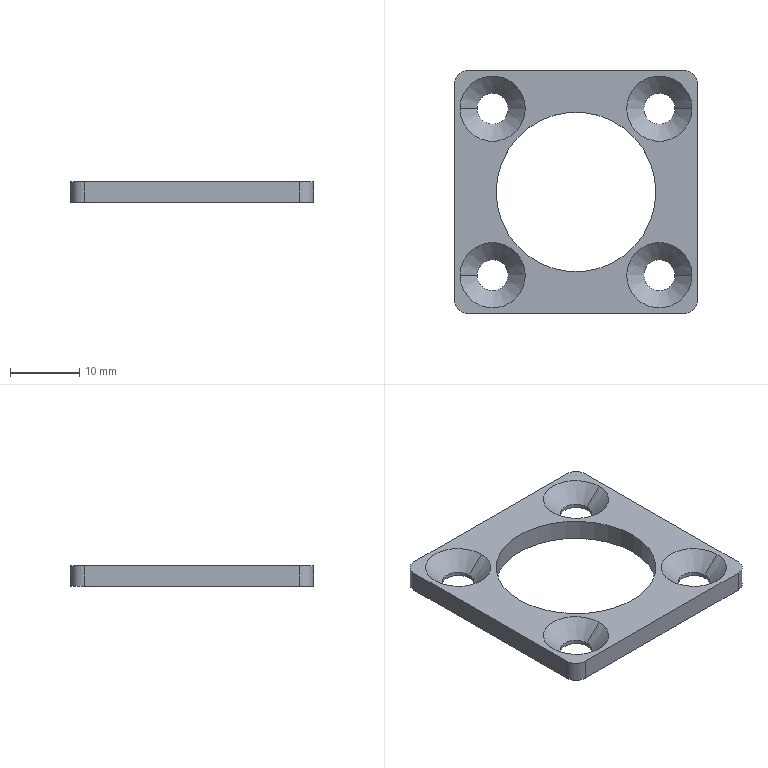Part | NX | features BREP 1 | 1 solid | 28 faces | box 35 x 35 x 3 mm | volume 1996 mm3 | cylinder 14 | cone 8 | plane 6 | commonest cylinder face diameters 4.5 x8 4 x4 23 x2
STEP:
#1=CARTESIAN_POINT('',(7.3,12.,3.));
#2=VERTEX_POINT('',#1);
#3=CARTESIAN_POINT('',(9.75,12.,0.55));
#4=VERTEX_POINT('',#3);
#5=CARTESIAN_POINT('',(7.3,12.,3.));
#6=DIRECTION('',(-0.7071,0.,0.7071));
#7=VECTOR('',#6,1000.);
#8=LINE('',#5,#7);
#9=EDGE_CURVE('',#2,#4,#8,.F.);
#10=ORIENTED_EDGE('',*,*,#9,.T.);
#11=CARTESIAN_POINT('',(14.25,12.,0.55));
#12=VERTEX_POINT('',#11);
#13=CARTESIAN_POINT('',(12.,12.,0.55));
#14=DIRECTION('',(0.,0.,1.));
#15=DIRECTION('',(1.,0.,0.));
#16=AXIS2_PLACEMENT_3D('',#13,#14,#15);
#17=CIRCLE('',#16,2.25);
#18=EDGE_CURVE('',#12,#4,#17,.T.);
#19=ORIENTED_EDGE('',*,*,#18,.F.);
#20=CARTESIAN_POINT('',(16.7,12.,3.));
#21=VERTEX_POINT('',#20);
#22=CARTESIAN_POINT('',(16.7,12.,3.));
#23=DIRECTION('',(0.7071,0.,0.7071));
#24=VECTOR('',#23,1000.);
#25=LINE('',#22,#24);
#26=EDGE_CURVE('',#21,#12,#25,.F.);
#27=ORIENTED_EDGE('',*,*,#26,.F.);
#28=CARTESIAN_POINT('',(12.,12.,3.));
#29=DIRECTION('',(0.,0.,1.));
#30=DIRECTION('',(1.,0.,0.));
#31=AXIS2_PLACEMENT_3D('',#28,#29,#30);
#32=CIRCLE('',#31,4.7);
#33=EDGE_CURVE('',#21,#2,#32,.T.);
#34=ORIENTED_EDGE('',*,*,#33,.T.);
#35=EDGE_LOOP('',(#10,#19,#27,#34));
#36=FACE_BOUND('',#35,.T.);
#37=CARTESIAN_POINT('',(12.,12.,3.));
#38=DIRECTION('',(0.,0.,1.));
#39=DIRECTION('',(1.,0.,0.));
#40=AXIS2_PLACEMENT_3D('',#37,#38,#39);
#41=CONICAL_SURFACE('',#40,4.7,0.7854);
#42=ADVANCED_FACE('',(#36),#41,.F.);
#43=CARTESIAN_POINT('',(9.75,12.,0.));
#44=VERTEX_POINT('',#43);
#45=CARTESIAN_POINT('',(9.75,12.,3.));
#46=DIRECTION('',(0.,0.,1.));
#47=VECTOR('',#46,1000.);
#48=LINE('',#45,#47);
#49=EDGE_CURVE('',#4,#44,#48,.F.);
#50=ORIENTED_EDGE('',*,*,#49,.T.);
#51=CARTESIAN_POINT('',(14.25,12.,0.));
#52=VERTEX_POINT('',#51);
#53=CARTESIAN_POINT('',(12.,12.,0.));
#54=DIRECTION('',(0.,0.,1.));
#55=DIRECTION('',(1.,0.,0.));
#56=AXIS2_PLACEMENT_3D('',#53,#54,#55);
#57=CIRCLE('',#56,2.25);
#58=EDGE_CURVE('',#52,#44,#57,.T.);
#59=ORIENTED_EDGE('',*,*,#58,.F.);
#60=CARTESIAN_POINT('',(14.25,12.,3.));
#61=DIRECTION('',(0.,0.,1.));
#62=VECTOR('',#61,1000.);
#63=LINE('',#60,#62);
#64=EDGE_CURVE('',#12,#52,#63,.F.);
#65=ORIENTED_EDGE('',*,*,#64,.F.);
#66=ORIENTED_EDGE('',*,*,#18,.T.);
#67=EDGE_LOOP('',(#50,#59,#65,#66));
#68=FACE_BOUND('',#67,.T.);
#69=CARTESIAN_POINT('',(12.,12.,3.));
#70=DIRECTION('',(0.,0.,1.));
#71=DIRECTION('',(1.,0.,0.));
#72=AXIS2_PLACEMENT_3D('',#69,#70,#71);
#73=CYLINDRICAL_SURFACE('',#72,2.25);
#74=ADVANCED_FACE('',(#68),#73,.F.);
#75=CARTESIAN_POINT('',(-16.7,-12.,3.));
#76=VERTEX_POINT('',#75);
#77=CARTESIAN_POINT('',(-14.25,-12.,0.55));
#78=VERTEX_POINT('',#77);
#79=CARTESIAN_POINT('',(-16.7,-12.,3.));
#80=DIRECTION('',(-0.7071,0.,0.7071));
#81=VECTOR('',#80,1000.);
#82=LINE('',#79,#81);
#83=EDGE_CURVE('',#76,#78,#82,.F.);
#84=ORIENTED_EDGE('',*,*,#83,.T.);
#85=CARTESIAN_POINT('',(-9.75,-12.,0.55));
#86=VERTEX_POINT('',#85);
#87=CARTESIAN_POINT('',(-12.,-12.,0.55));
#88=DIRECTION('',(0.,0.,1.));
#89=DIRECTION('',(1.,0.,0.));
#90=AXIS2_PLACEMENT_3D('',#87,#88,#89);
#91=CIRCLE('',#90,2.25);
#92=EDGE_CURVE('',#86,#78,#91,.T.);
#93=ORIENTED_EDGE('',*,*,#92,.F.);
#94=CARTESIAN_POINT('',(-7.3,-12.,3.));
#95=VERTEX_POINT('',#94);
#96=CARTESIAN_POINT('',(-7.3,-12.,3.));
#97=DIRECTION('',(0.7071,0.,0.7071));
#98=VECTOR('',#97,1000.);
#99=LINE('',#96,#98);
#100=EDGE_CURVE('',#95,#86,#99,.F.);
#101=ORIENTED_EDGE('',*,*,#100,.F.);
#102=CARTESIAN_POINT('',(-12.,-12.,3.));
#103=DIRECTION('',(0.,0.,1.));
#104=DIRECTION('',(1.,0.,0.));
#105=AXIS2_PLACEMENT_3D('',#102,#103,#104);
#106=CIRCLE('',#105,4.7);
#107=EDGE_CURVE('',#95,#76,#106,.T.);
#108=ORIENTED_EDGE('',*,*,#107,.T.);
#109=EDGE_LOOP('',(#84,#93,#101,#108));
#110=FACE_BOUND('',#109,.T.);
#111=CARTESIAN_POINT('',(-12.,-12.,3.));
#112=DIRECTION('',(0.,0.,1.));
#113=DIRECTION('',(1.,0.,0.));
#114=AXIS2_PLACEMENT_3D('',#111,#112,#113);
#115=CONICAL_SURFACE('',#114,4.7,0.7854);
#116=ADVANCED_FACE('',(#110),#115,.F.);
#117=CARTESIAN_POINT('',(-14.25,-12.,0.));
#118=VERTEX_POINT('',#117);
#119=CARTESIAN_POINT('',(-14.25,-12.,3.));
#120=DIRECTION('',(0.,0.,1.));
#121=VECTOR('',#120,1000.);
#122=LINE('',#119,#121);
#123=EDGE_CURVE('',#78,#118,#122,.F.);
#124=ORIENTED_EDGE('',*,*,#123,.T.);
#125=CARTESIAN_POINT('',(-9.75,-12.,0.));
#126=VERTEX_POINT('',#125);
#127=CARTESIAN_POINT('',(-12.,-12.,0.));
#128=DIRECTION('',(0.,0.,1.));
#129=DIRECTION('',(1.,0.,0.));
#130=AXIS2_PLACEMENT_3D('',#127,#128,#129);
#131=CIRCLE('',#130,2.25);
#132=EDGE_CURVE('',#126,#118,#131,.T.);
#133=ORIENTED_EDGE('',*,*,#132,.F.);
#134=CARTESIAN_POINT('',(-9.75,-12.,3.));
#135=DIRECTION('',(0.,0.,1.));
#136=VECTOR('',#135,1000.);
#137=LINE('',#134,#136);
#138=EDGE_CURVE('',#86,#126,#137,.F.);
#139=ORIENTED_EDGE('',*,*,#138,.F.);
#140=ORIENTED_EDGE('',*,*,#92,.T.);
#141=EDGE_LOOP('',(#124,#133,#139,#140));
#142=FACE_BOUND('',#141,.T.);
#143=CARTESIAN_POINT('',(-12.,-12.,3.));
#144=DIRECTION('',(0.,0.,1.));
#145=DIRECTION('',(1.,0.,0.));
#146=AXIS2_PLACEMENT_3D('',#143,#144,#145);
#147=CYLINDRICAL_SURFACE('',#146,2.25);
#148=ADVANCED_FACE('',(#142),#147,.F.);
#149=CARTESIAN_POINT('',(-16.7,12.,3.));
#150=VERTEX_POINT('',#149);
#151=CARTESIAN_POINT('',(-14.25,12.,0.55));
#152=VERTEX_POINT('',#151);
#153=CARTESIAN_POINT('',(-16.7,12.,3.));
#154=DIRECTION('',(-0.7071,0.,0.7071));
#155=VECTOR('',#154,1000.);
#156=LINE('',#153,#155);
#157=EDGE_CURVE('',#150,#152,#156,.F.);
#158=ORIENTED_EDGE('',*,*,#157,.T.);
#159=CARTESIAN_POINT('',(-9.75,12.,0.55));
#160=VERTEX_POINT('',#159);
#161=CARTESIAN_POINT('',(-12.,12.,0.55));
#162=DIRECTION('',(0.,0.,1.));
#163=DIRECTION('',(1.,0.,0.));
#164=AXIS2_PLACEMENT_3D('',#161,#162,#163);
#165=CIRCLE('',#164,2.25);
#166=EDGE_CURVE('',#160,#152,#165,.T.);
#167=ORIENTED_EDGE('',*,*,#166,.F.);
#168=CARTESIAN_POINT('',(-7.3,12.,3.));
#169=VERTEX_POINT('',#168);
#170=CARTESIAN_POINT('',(-7.3,12.,3.));
#171=DIRECTION('',(0.7071,0.,0.7071));
#172=VECTOR('',#171,1000.);
#173=LINE('',#170,#172);
#174=EDGE_CURVE('',#169,#160,#173,.F.);
#175=ORIENTED_EDGE('',*,*,#174,.F.);
#176=CARTESIAN_POINT('',(-12.,12.,3.));
#177=DIRECTION('',(0.,0.,1.));
#178=DIRECTION('',(1.,0.,0.));
#179=AXIS2_PLACEMENT_3D('',#176,#177,#178);
#180=CIRCLE('',#179,4.7);
#181=EDGE_CURVE('',#169,#150,#180,.T.);
#182=ORIENTED_EDGE('',*,*,#181,.T.);
#183=EDGE_LOOP('',(#158,#167,#175,#182));
#184=FACE_BOUND('',#183,.T.);
#185=CARTESIAN_POINT('',(-12.,12.,3.));
#186=DIRECTION('',(0.,0.,1.));
#187=DIRECTION('',(1.,0.,0.));
#188=AXIS2_PLACEMENT_3D('',#185,#186,#187);
#189=CONICAL_SURFACE('',#188,4.7,0.7854);
#190=ADVANCED_FACE('',(#184),#189,.F.);
#191=CARTESIAN_POINT('',(-14.25,12.,0.));
#192=VERTEX_POINT('',#191);
#193=CARTESIAN_POINT('',(-14.25,12.,3.));
#194=DIRECTION('',(0.,0.,1.));
#195=VECTOR('',#194,1000.);
#196=LINE('',#193,#195);
#197=EDGE_CURVE('',#152,#192,#196,.F.);
#198=ORIENTED_EDGE('',*,*,#197,.T.);
#199=CARTESIAN_POINT('',(-9.75,12.,0.));
#200=VERTEX_POINT('',#199);
#201=CARTESIAN_POINT('',(-12.,12.,0.));
#202=DIRECTION('',(0.,0.,1.));
#203=DIRECTION('',(1.,0.,0.));
#204=AXIS2_PLACEMENT_3D('',#201,#202,#203);
#205=CIRCLE('',#204,2.25);
#206=EDGE_CURVE('',#200,#192,#205,.T.);
#207=ORIENTED_EDGE('',*,*,#206,.F.);
#208=CARTESIAN_POINT('',(-9.75,12.,3.));
#209=DIRECTION('',(0.,0.,1.));
#210=VECTOR('',#209,1000.);
#211=LINE('',#208,#210);
#212=EDGE_CURVE('',#160,#200,#211,.F.);
#213=ORIENTED_EDGE('',*,*,#212,.F.);
#214=ORIENTED_EDGE('',*,*,#166,.T.);
#215=EDGE_LOOP('',(#198,#207,#213,#214));
#216=FACE_BOUND('',#215,.T.);
#217=CARTESIAN_POINT('',(-12.,12.,3.));
#218=DIRECTION('',(0.,0.,1.));
#219=DIRECTION('',(1.,0.,0.));
#220=AXIS2_PLACEMENT_3D('',#217,#218,#219);
#221=CYLINDRICAL_SURFACE('',#220,2.25);
#222=ADVANCED_FACE('',(#216),#221,.F.);
#223=CARTESIAN_POINT('',(7.3,-12.,3.));
#224=VERTEX_POINT('',#223);
#225=CARTESIAN_POINT('',(9.75,-12.,0.55));
#226=VERTEX_POINT('',#225);
#227=CARTESIAN_POINT('',(7.3,-12.,3.));
#228=DIRECTION('',(-0.7071,0.,0.7071));
#229=VECTOR('',#228,1000.);
#230=LINE('',#227,#229);
#231=EDGE_CURVE('',#224,#226,#230,.F.);
#232=ORIENTED_EDGE('',*,*,#231,.T.);
#233=CARTESIAN_POINT('',(14.25,-12.,0.55));
#234=VERTEX_POINT('',#233);
#235=CARTESIAN_POINT('',(12.,-12.,0.55));
#236=DIRECTION('',(0.,0.,1.));
#237=DIRECTION('',(1.,0.,0.));
#238=AXIS2_PLACEMENT_3D('',#235,#236,#237);
#239=CIRCLE('',#238,2.25);
#240=EDGE_CURVE('',#234,#226,#239,.T.);
#241=ORIENTED_EDGE('',*,*,#240,.F.);
#242=CARTESIAN_POINT('',(16.7,-12.,3.));
#243=VERTEX_POINT('',#242);
#244=CARTESIAN_POINT('',(16.7,-12.,3.));
#245=DIRECTION('',(0.7071,0.,0.7071));
#246=VECTOR('',#245,1000.);
#247=LINE('',#244,#246);
#248=EDGE_CURVE('',#243,#234,#247,.F.);
#249=ORIENTED_EDGE('',*,*,#248,.F.);
#250=CARTESIAN_POINT('',(12.,-12.,3.));
#251=DIRECTION('',(0.,0.,1.));
#252=DIRECTION('',(1.,0.,0.));
#253=AXIS2_PLACEMENT_3D('',#250,#251,#252);
#254=CIRCLE('',#253,4.7);
#255=EDGE_CURVE('',#243,#224,#254,.T.);
#256=ORIENTED_EDGE('',*,*,#255,.T.);
#257=EDGE_LOOP('',(#232,#241,#249,#256));
#258=FACE_BOUND('',#257,.T.);
#259=CARTESIAN_POINT('',(12.,-12.,3.));
#260=DIRECTION('',(0.,0.,1.));
#261=DIRECTION('',(1.,0.,0.));
#262=AXIS2_PLACEMENT_3D('',#259,#260,#261);
#263=CONICAL_SURFACE('',#262,4.7,0.7854);
#264=ADVANCED_FACE('',(#258),#263,.F.);
#265=CARTESIAN_POINT('',(9.75,-12.,0.));
#266=VERTEX_POINT('',#265);
#267=CARTESIAN_POINT('',(9.75,-12.,3.));
#268=DIRECTION('',(0.,0.,1.));
#269=VECTOR('',#268,1000.);
#270=LINE('',#267,#269);
#271=EDGE_CURVE('',#226,#266,#270,.F.);
#272=ORIENTED_EDGE('',*,*,#271,.T.);
#273=CARTESIAN_POINT('',(14.25,-12.,0.));
#274=VERTEX_POINT('',#273);
#275=CARTESIAN_POINT('',(12.,-12.,0.));
#276=DIRECTION('',(0.,0.,1.));
#277=DIRECTION('',(1.,0.,0.));
#278=AXIS2_PLACEMENT_3D('',#275,#276,#277);
#279=CIRCLE('',#278,2.25);
#280=EDGE_CURVE('',#274,#266,#279,.T.);
#281=ORIENTED_EDGE('',*,*,#280,.F.);
#282=CARTESIAN_POINT('',(14.25,-12.,3.));
#283=DIRECTION('',(0.,0.,1.));
#284=VECTOR('',#283,1000.);
#285=LINE('',#282,#284);
#286=EDGE_CURVE('',#234,#274,#285,.F.);
#287=ORIENTED_EDGE('',*,*,#286,.F.);
#288=ORIENTED_EDGE('',*,*,#240,.T.);
#289=EDGE_LOOP('',(#272,#281,#287,#288));
#290=FACE_BOUND('',#289,.T.);
#291=CARTESIAN_POINT('',(12.,-12.,3.));
#292=DIRECTION('',(0.,0.,1.));
#293=DIRECTION('',(1.,0.,0.));
#294=AXIS2_PLACEMENT_3D('',#291,#292,#293);
#295=CYLINDRICAL_SURFACE('',#294,2.25);
#296=ADVANCED_FACE('',(#290),#295,.F.);
#297=CARTESIAN_POINT('',(11.5,0.,3.));
#298=VERTEX_POINT('',#297);
#299=CARTESIAN_POINT('',(11.5,0.,0.));
#300=VERTEX_POINT('',#299);
#301=CARTESIAN_POINT('',(11.5,0.,3.));
#302=DIRECTION('',(0.,0.,-1.));
#303=VECTOR('',#302,1000.);
#304=LINE('',#301,#303);
#305=EDGE_CURVE('',#298,#300,#304,.T.);
#306=ORIENTED_EDGE('',*,*,#305,.F.);
#307=CARTESIAN_POINT('',(-11.5,0.,3.));
#308=VERTEX_POINT('',#307);
#309=CARTESIAN_POINT('',(0.,0.,3.));
#310=DIRECTION('',(0.,0.,1.));
#311=DIRECTION('',(1.,0.,0.));
#312=AXIS2_PLACEMENT_3D('',#309,#310,#311);
#313=CIRCLE('',#312,11.5);
#314=EDGE_CURVE('',#298,#308,#313,.T.);
#315=ORIENTED_EDGE('',*,*,#314,.T.);
#316=CARTESIAN_POINT('',(-11.5,0.,0.));
#317=VERTEX_POINT('',#316);
#318=CARTESIAN_POINT('',(-11.5,0.,3.));
#319=DIRECTION('',(0.,0.,-1.));
#320=VECTOR('',#319,1000.);
#321=LINE('',#318,#320);
#322=EDGE_CURVE('',#308,#317,#321,.T.);
#323=ORIENTED_EDGE('',*,*,#322,.T.);
#324=CARTESIAN_POINT('',(0.,0.,0.));
#325=DIRECTION('',(0.,0.,1.));
#326=DIRECTION('',(1.,0.,0.));
#327=AXIS2_PLACEMENT_3D('',#324,#325,#326);
#328=CIRCLE('',#327,11.5);
#329=EDGE_CURVE('',#300,#317,#328,.T.);
#330=ORIENTED_EDGE('',*,*,#329,.F.);
#331=EDGE_LOOP('',(#306,#315,#323,#330));
#332=FACE_BOUND('',#331,.T.);
#333=CARTESIAN_POINT('',(0.,0.,3.));
#334=DIRECTION('',(0.,0.,-1.));
#335=DIRECTION('',(-1.,0.,0.));
#336=AXIS2_PLACEMENT_3D('',#333,#334,#335);
#337=CYLINDRICAL_SURFACE('',#336,11.5);
#338=ADVANCED_FACE('',(#332),#337,.F.);
#339=CARTESIAN_POINT('',(17.5,-15.5,0.));
#340=VERTEX_POINT('',#339);
#341=CARTESIAN_POINT('',(17.5,15.5,0.));
#342=VERTEX_POINT('',#341);
#343=CARTESIAN_POINT('',(17.5,-15.5,0.));
#344=DIRECTION('',(0.,1.,0.));
#345=VECTOR('',#344,1000.);
#346=LINE('',#343,#345);
#347=EDGE_CURVE('',#340,#342,#346,.T.);
#348=ORIENTED_EDGE('',*,*,#347,.T.);
#349=CARTESIAN_POINT('',(17.5,15.5,3.));
#350=VERTEX_POINT('',#349);
#351=CARTESIAN_POINT('',(17.5,15.5,3.));
#352=DIRECTION('',(0.,0.,-1.));
#353=VECTOR('',#352,1000.);
#354=LINE('',#351,#353);
#355=EDGE_CURVE('',#350,#342,#354,.T.);
#356=ORIENTED_EDGE('',*,*,#355,.F.);
#357=CARTESIAN_POINT('',(17.5,-15.5,3.));
#358=VERTEX_POINT('',#357);
#359=CARTESIAN_POINT('',(17.5,-15.5,3.));
#360=DIRECTION('',(0.,1.,0.));
#361=VECTOR('',#360,1000.);
#362=LINE('',#359,#361);
#363=EDGE_CURVE('',#358,#350,#362,.T.);
#364=ORIENTED_EDGE('',*,*,#363,.F.);
#365=CARTESIAN_POINT('',(17.5,-15.5,3.));
#366=DIRECTION('',(0.,0.,-1.));
#367=VECTOR('',#366,1000.);
#368=LINE('',#365,#367);
#369=EDGE_CURVE('',#358,#340,#368,.T.);
#370=ORIENTED_EDGE('',*,*,#369,.T.);
#371=EDGE_LOOP('',(#348,#356,#364,#370));
#372=FACE_BOUND('',#371,.T.);
#373=CARTESIAN_POINT('',(17.5,-15.5,3.));
#374=DIRECTION('',(-1.,0.,0.));
#375=DIRECTION('',(0.,0.,1.));
#376=AXIS2_PLACEMENT_3D('',#373,#374,#375);
#377=PLANE('',#376);
#378=ADVANCED_FACE('',(#372),#377,.F.);
#379=CARTESIAN_POINT('',(15.5,-17.5,0.));
#380=VERTEX_POINT('',#379);
#381=CARTESIAN_POINT('',(15.5,-15.5,0.));
#382=DIRECTION('',(0.,0.,1.));
#383=DIRECTION('',(1.,0.,0.));
#384=AXIS2_PLACEMENT_3D('',#381,#382,#383);
#385=CIRCLE('',#384,2.);
#386=EDGE_CURVE('',#380,#340,#385,.T.);
#387=ORIENTED_EDGE('',*,*,#386,.T.);
#388=ORIENTED_EDGE('',*,*,#369,.F.);
#389=CARTESIAN_POINT('',(15.5,-17.5,3.));
#390=VERTEX_POINT('',#389);
#391=CARTESIAN_POINT('',(15.5,-15.5,3.));
#392=DIRECTION('',(0.,0.,1.));
#393=DIRECTION('',(1.,0.,0.));
#394=AXIS2_PLACEMENT_3D('',#391,#392,#393);
#395=CIRCLE('',#394,2.);
#396=EDGE_CURVE('',#390,#358,#395,.T.);
#397=ORIENTED_EDGE('',*,*,#396,.F.);
#398=CARTESIAN_POINT('',(15.5,-17.5,3.));
#399=DIRECTION('',(0.,0.,-1.));
#400=VECTOR('',#399,1000.);
#401=LINE('',#398,#400);
#402=EDGE_CURVE('',#390,#380,#401,.T.);
#403=ORIENTED_EDGE('',*,*,#402,.T.);
#404=EDGE_LOOP('',(#387,#388,#397,#403));
#405=FACE_BOUND('',#404,.T.);
#406=CARTESIAN_POINT('',(15.5,-15.5,3.));
#407=DIRECTION('',(0.,0.,-1.));
#408=DIRECTION('',(-1.,0.,0.));
#409=AXIS2_PLACEMENT_3D('',#406,#407,#408);
#410=CYLINDRICAL_SURFACE('',#409,2.);
#411=ADVANCED_FACE('',(#405),#410,.T.);
#412=CARTESIAN_POINT('',(-15.5,-17.5,0.));
#413=VERTEX_POINT('',#412);
#414=CARTESIAN_POINT('',(-15.5,-17.5,0.));
#415=DIRECTION('',(1.,0.,0.));
#416=VECTOR('',#415,1000.);
#417=LINE('',#414,#416);
#418=EDGE_CURVE('',#413,#380,#417,.T.);
#419=ORIENTED_EDGE('',*,*,#418,.T.);
#420=ORIENTED_EDGE('',*,*,#402,.F.);
#421=CARTESIAN_POINT('',(-15.5,-17.5,3.));
#422=VERTEX_POINT('',#421);
#423=CARTESIAN_POINT('',(-15.5,-17.5,3.));
#424=DIRECTION('',(1.,0.,0.));
#425=VECTOR('',#424,1000.);
#426=LINE('',#423,#425);
#427=EDGE_CURVE('',#422,#390,#426,.T.);
#428=ORIENTED_EDGE('',*,*,#427,.F.);
#429=CARTESIAN_POINT('',(-15.5,-17.5,3.));
#430=DIRECTION('',(0.,0.,-1.));
#431=VECTOR('',#430,1000.);
#432=LINE('',#429,#431);
#433=EDGE_CURVE('',#422,#413,#432,.T.);
#434=ORIENTED_EDGE('',*,*,#433,.T.);
#435=EDGE_LOOP('',(#419,#420,#428,#434));
#436=FACE_BOUND('',#435,.T.);
#437=CARTESIAN_POINT('',(-15.5,-17.5,3.));
#438=DIRECTION('',(0.,1.,0.));
#439=DIRECTION('',(0.,0.,1.));
#440=AXIS2_PLACEMENT_3D('',#437,#438,#439);
#441=PLANE('',#440);
#442=ADVANCED_FACE('',(#436),#441,.F.);
#443=CARTESIAN_POINT('',(-17.5,-15.5,0.));
#444=VERTEX_POINT('',#443);
#445=CARTESIAN_POINT('',(-15.5,-15.5,0.));
#446=DIRECTION('',(0.,0.,1.));
#447=DIRECTION('',(-1.,0.,0.));
#448=AXIS2_PLACEMENT_3D('',#445,#446,#447);
#449=CIRCLE('',#448,2.);
#450=EDGE_CURVE('',#444,#413,#449,.T.);
#451=ORIENTED_EDGE('',*,*,#450,.T.);
#452=ORIENTED_EDGE('',*,*,#433,.F.);
#453=CARTESIAN_POINT('',(-17.5,-15.5,3.));
#454=VERTEX_POINT('',#453);
#455=CARTESIAN_POINT('',(-15.5,-15.5,3.));
#456=DIRECTION('',(0.,0.,1.));
#457=DIRECTION('',(-1.,0.,0.));
#458=AXIS2_PLACEMENT_3D('',#455,#456,#457);
#459=CIRCLE('',#458,2.);
#460=EDGE_CURVE('',#454,#422,#459,.T.);
#461=ORIENTED_EDGE('',*,*,#460,.F.);
#462=CARTESIAN_POINT('',(-17.5,-15.5,3.));
#463=DIRECTION('',(0.,0.,-1.));
#464=VECTOR('',#463,1000.);
#465=LINE('',#462,#464);
#466=EDGE_CURVE('',#454,#444,#465,.T.);
#467=ORIENTED_EDGE('',*,*,#466,.T.);
#468=EDGE_LOOP('',(#451,#452,#461,#467));
#469=FACE_BOUND('',#468,.T.);
#470=CARTESIAN_POINT('',(-15.5,-15.5,3.));
#471=DIRECTION('',(0.,0.,-1.));
#472=DIRECTION('',(-1.,0.,0.));
#473=AXIS2_PLACEMENT_3D('',#470,#471,#472);
#474=CYLINDRICAL_SURFACE('',#473,2.);
#475=ADVANCED_FACE('',(#469),#474,.T.);
#476=CARTESIAN_POINT('',(-17.5,15.5,0.));
#477=VERTEX_POINT('',#476);
#478=CARTESIAN_POINT('',(-17.5,-15.5,0.));
#479=DIRECTION('',(0.,-1.,0.));
#480=VECTOR('',#479,1000.);
#481=LINE('',#478,#480);
#482=EDGE_CURVE('',#477,#444,#481,.T.);
#483=ORIENTED_EDGE('',*,*,#482,.T.);
#484=ORIENTED_EDGE('',*,*,#466,.F.);
#485=CARTESIAN_POINT('',(-17.5,15.5,3.));
#486=VERTEX_POINT('',#485);
#487=CARTESIAN_POINT('',(-17.5,-15.5,3.));
#488=DIRECTION('',(0.,-1.,0.));
#489=VECTOR('',#488,1000.);
#490=LINE('',#487,#489);
#491=EDGE_CURVE('',#486,#454,#490,.T.);
#492=ORIENTED_EDGE('',*,*,#491,.F.);
#493=CARTESIAN_POINT('',(-17.5,15.5,3.));
#494=DIRECTION('',(0.,0.,-1.));
#495=VECTOR('',#494,1000.);
#496=LINE('',#493,#495);
#497=EDGE_CURVE('',#486,#477,#496,.T.);
#498=ORIENTED_EDGE('',*,*,#497,.T.);
#499=EDGE_LOOP('',(#483,#484,#492,#498));
#500=FACE_BOUND('',#499,.T.);
#501=CARTESIAN_POINT('',(-17.5,-15.5,3.));
#502=DIRECTION('',(1.,0.,0.));
#503=DIRECTION('',(0.,0.,-1.));
#504=AXIS2_PLACEMENT_3D('',#501,#502,#503);
#505=PLANE('',#504);
#506=ADVANCED_FACE('',(#500),#505,.F.);
#507=CARTESIAN_POINT('',(-15.5,17.5,0.));
#508=VERTEX_POINT('',#507);
#509=CARTESIAN_POINT('',(-15.5,15.5,0.));
#510=DIRECTION('',(0.,0.,1.));
#511=DIRECTION('',(-1.,0.,0.));
#512=AXIS2_PLACEMENT_3D('',#509,#510,#511);
#513=CIRCLE('',#512,2.);
#514=EDGE_CURVE('',#508,#477,#513,.T.);
#515=ORIENTED_EDGE('',*,*,#514,.T.);
#516=ORIENTED_EDGE('',*,*,#497,.F.);
#517=CARTESIAN_POINT('',(-15.5,17.5,3.));
#518=VERTEX_POINT('',#517);
#519=CARTESIAN_POINT('',(-15.5,15.5,3.));
#520=DIRECTION('',(0.,0.,1.));
#521=DIRECTION('',(-1.,0.,0.));
#522=AXIS2_PLACEMENT_3D('',#519,#520,#521);
#523=CIRCLE('',#522,2.);
#524=EDGE_CURVE('',#518,#486,#523,.T.);
#525=ORIENTED_EDGE('',*,*,#524,.F.);
#526=CARTESIAN_POINT('',(-15.5,17.5,3.));
#527=DIRECTION('',(0.,0.,-1.));
#528=VECTOR('',#527,1000.);
#529=LINE('',#526,#528);
#530=EDGE_CURVE('',#518,#508,#529,.T.);
#531=ORIENTED_EDGE('',*,*,#530,.T.);
#532=EDGE_LOOP('',(#515,#516,#525,#531));
#533=FACE_BOUND('',#532,.T.);
#534=CARTESIAN_POINT('',(-15.5,15.5,3.));
#535=DIRECTION('',(0.,0.,-1.));
#536=DIRECTION('',(-1.,0.,0.));
#537=AXIS2_PLACEMENT_3D('',#534,#535,#536);
#538=CYLINDRICAL_SURFACE('',#537,2.);
#539=ADVANCED_FACE('',(#533),#538,.T.);
#540=CARTESIAN_POINT('',(15.5,17.5,0.));
#541=VERTEX_POINT('',#540);
#542=CARTESIAN_POINT('',(-15.5,17.5,0.));
#543=DIRECTION('',(-1.,0.,0.));
#544=VECTOR('',#543,1000.);
#545=LINE('',#542,#544);
#546=EDGE_CURVE('',#541,#508,#545,.T.);
#547=ORIENTED_EDGE('',*,*,#546,.T.);
#548=ORIENTED_EDGE('',*,*,#530,.F.);
#549=CARTESIAN_POINT('',(15.5,17.5,3.));
#550=VERTEX_POINT('',#549);
#551=CARTESIAN_POINT('',(-15.5,17.5,3.));
#552=DIRECTION('',(-1.,0.,0.));
#553=VECTOR('',#552,1000.);
#554=LINE('',#551,#553);
#555=EDGE_CURVE('',#550,#518,#554,.T.);
#556=ORIENTED_EDGE('',*,*,#555,.F.);
#557=CARTESIAN_POINT('',(15.5,17.5,3.));
#558=DIRECTION('',(0.,0.,-1.));
#559=VECTOR('',#558,1000.);
#560=LINE('',#557,#559);
#561=EDGE_CURVE('',#550,#541,#560,.T.);
#562=ORIENTED_EDGE('',*,*,#561,.T.);
#563=EDGE_LOOP('',(#547,#548,#556,#562));
#564=FACE_BOUND('',#563,.T.);
#565=CARTESIAN_POINT('',(-15.5,17.5,3.));
#566=DIRECTION('',(0.,-1.,0.));
#567=DIRECTION('',(0.,0.,-1.));
#568=AXIS2_PLACEMENT_3D('',#565,#566,#567);
#569=PLANE('',#568);
#570=ADVANCED_FACE('',(#564),#569,.F.);
#571=CARTESIAN_POINT('',(15.5,15.5,0.));
#572=DIRECTION('',(0.,0.,1.));
#573=DIRECTION('',(1.,0.,0.));
#574=AXIS2_PLACEMENT_3D('',#571,#572,#573);
#575=CIRCLE('',#574,2.);
#576=EDGE_CURVE('',#342,#541,#575,.T.);
#577=ORIENTED_EDGE('',*,*,#576,.T.);
#578=ORIENTED_EDGE('',*,*,#561,.F.);
#579=CARTESIAN_POINT('',(15.5,15.5,3.));
#580=DIRECTION('',(0.,0.,1.));
#581=DIRECTION('',(1.,0.,0.));
#582=AXIS2_PLACEMENT_3D('',#579,#580,#581);
#583=CIRCLE('',#582,2.);
#584=EDGE_CURVE('',#350,#550,#583,.T.);
#585=ORIENTED_EDGE('',*,*,#584,.F.);
#586=ORIENTED_EDGE('',*,*,#355,.T.);
#587=EDGE_LOOP('',(#577,#578,#585,#586));
#588=FACE_BOUND('',#587,.T.);
#589=CARTESIAN_POINT('',(15.5,15.5,3.));
#590=DIRECTION('',(0.,0.,-1.));
#591=DIRECTION('',(-1.,0.,0.));
#592=AXIS2_PLACEMENT_3D('',#589,#590,#591);
#593=CYLINDRICAL_SURFACE('',#592,2.);
#594=ADVANCED_FACE('',(#588),#593,.T.);
#595=CARTESIAN_POINT('',(0.,0.,0.));
#596=DIRECTION('',(0.,0.,1.));
#597=DIRECTION('',(1.,0.,0.));
#598=AXIS2_PLACEMENT_3D('',#595,#596,#597);
#599=CIRCLE('',#598,11.5);
#600=EDGE_CURVE('',#317,#300,#599,.T.);
#601=ORIENTED_EDGE('',*,*,#600,.T.);
#602=ORIENTED_EDGE('',*,*,#329,.T.);
#603=EDGE_LOOP('',(#601,#602));
#604=FACE_BOUND('',#603,.T.);
#605=ORIENTED_EDGE('',*,*,#576,.F.);
#606=ORIENTED_EDGE('',*,*,#347,.F.);
#607=ORIENTED_EDGE('',*,*,#386,.F.);
#608=ORIENTED_EDGE('',*,*,#418,.F.);
#609=ORIENTED_EDGE('',*,*,#450,.F.);
#610=ORIENTED_EDGE('',*,*,#482,.F.);
#611=ORIENTED_EDGE('',*,*,#514,.F.);
#612=ORIENTED_EDGE('',*,*,#546,.F.);
#613=EDGE_LOOP('',(#605,#606,#607,#608,#609,#610,#611,#612));
#614=FACE_BOUND('',#613,.T.);
#615=ORIENTED_EDGE('',*,*,#280,.T.);
#616=CARTESIAN_POINT('',(12.,-12.,0.));
#617=DIRECTION('',(0.,0.,1.));
#618=DIRECTION('',(1.,0.,0.));
#619=AXIS2_PLACEMENT_3D('',#616,#617,#618);
#620=CIRCLE('',#619,2.25);
#621=EDGE_CURVE('',#266,#274,#620,.T.);
#622=ORIENTED_EDGE('',*,*,#621,.T.);
#623=EDGE_LOOP('',(#615,#622));
#624=FACE_BOUND('',#623,.T.);
#625=ORIENTED_EDGE('',*,*,#206,.T.);
#626=CARTESIAN_POINT('',(-12.,12.,0.));
#627=DIRECTION('',(0.,0.,1.));
#628=DIRECTION('',(1.,0.,0.));
#629=AXIS2_PLACEMENT_3D('',#626,#627,#628);
#630=CIRCLE('',#629,2.25);
#631=EDGE_CURVE('',#192,#200,#630,.T.);
#632=ORIENTED_EDGE('',*,*,#631,.T.);
#633=EDGE_LOOP('',(#625,#632));
#634=FACE_BOUND('',#633,.T.);
#635=ORIENTED_EDGE('',*,*,#132,.T.);
#636=CARTESIAN_POINT('',(-12.,-12.,0.));
#637=DIRECTION('',(0.,0.,1.));
#638=DIRECTION('',(1.,0.,0.));
#639=AXIS2_PLACEMENT_3D('',#636,#637,#638);
#640=CIRCLE('',#639,2.25);
#641=EDGE_CURVE('',#118,#126,#640,.T.);
#642=ORIENTED_EDGE('',*,*,#641,.T.);
#643=EDGE_LOOP('',(#635,#642));
#644=FACE_BOUND('',#643,.T.);
#645=ORIENTED_EDGE('',*,*,#58,.T.);
#646=CARTESIAN_POINT('',(12.,12.,0.));
#647=DIRECTION('',(0.,0.,1.));
#648=DIRECTION('',(1.,0.,0.));
#649=AXIS2_PLACEMENT_3D('',#646,#647,#648);
#650=CIRCLE('',#649,2.25);
#651=EDGE_CURVE('',#44,#52,#650,.T.);
#652=ORIENTED_EDGE('',*,*,#651,.T.);
#653=EDGE_LOOP('',(#645,#652));
#654=FACE_BOUND('',#653,.T.);
#655=CARTESIAN_POINT('',(15.5,15.5,0.));
#656=DIRECTION('',(0.,0.,1.));
#657=DIRECTION('',(1.,0.,0.));
#658=AXIS2_PLACEMENT_3D('',#655,#656,#657);
#659=PLANE('',#658);
#660=ADVANCED_FACE('',(#604,#614,#624,#634,#644,#654),#659,.F.);
#661=CARTESIAN_POINT('',(0.,0.,3.));
#662=DIRECTION('',(0.,0.,1.));
#663=DIRECTION('',(1.,0.,0.));
#664=AXIS2_PLACEMENT_3D('',#661,#662,#663);
#665=CIRCLE('',#664,11.5);
#666=EDGE_CURVE('',#308,#298,#665,.T.);
#667=ORIENTED_EDGE('',*,*,#666,.F.);
#668=ORIENTED_EDGE('',*,*,#314,.F.);
#669=EDGE_LOOP('',(#667,#668));
#670=FACE_BOUND('',#669,.T.);
#671=ORIENTED_EDGE('',*,*,#584,.T.);
#672=ORIENTED_EDGE('',*,*,#555,.T.);
#673=ORIENTED_EDGE('',*,*,#524,.T.);
#674=ORIENTED_EDGE('',*,*,#491,.T.);
#675=ORIENTED_EDGE('',*,*,#460,.T.);
#676=ORIENTED_EDGE('',*,*,#427,.T.);
#677=ORIENTED_EDGE('',*,*,#396,.T.);
#678=ORIENTED_EDGE('',*,*,#363,.T.);
#679=EDGE_LOOP('',(#671,#672,#673,#674,#675,#676,#677,#678));
#680=FACE_BOUND('',#679,.T.);
#681=ORIENTED_EDGE('',*,*,#255,.F.);
#682=CARTESIAN_POINT('',(12.,-12.,3.));
#683=DIRECTION('',(0.,0.,1.));
#684=DIRECTION('',(1.,0.,0.));
#685=AXIS2_PLACEMENT_3D('',#682,#683,#684);
#686=CIRCLE('',#685,4.7);
#687=EDGE_CURVE('',#224,#243,#686,.T.);
#688=ORIENTED_EDGE('',*,*,#687,.F.);
#689=EDGE_LOOP('',(#681,#688));
#690=FACE_BOUND('',#689,.T.);
#691=ORIENTED_EDGE('',*,*,#181,.F.);
#692=CARTESIAN_POINT('',(-12.,12.,3.));
#693=DIRECTION('',(0.,0.,1.));
#694=DIRECTION('',(1.,0.,0.));
#695=AXIS2_PLACEMENT_3D('',#692,#693,#694);
#696=CIRCLE('',#695,4.7);
#697=EDGE_CURVE('',#150,#169,#696,.T.);
#698=ORIENTED_EDGE('',*,*,#697,.F.);
#699=EDGE_LOOP('',(#691,#698));
#700=FACE_BOUND('',#699,.T.);
#701=ORIENTED_EDGE('',*,*,#107,.F.);
#702=CARTESIAN_POINT('',(-12.,-12.,3.));
#703=DIRECTION('',(0.,0.,1.));
#704=DIRECTION('',(1.,0.,0.));
#705=AXIS2_PLACEMENT_3D('',#702,#703,#704);
#706=CIRCLE('',#705,4.7);
#707=EDGE_CURVE('',#76,#95,#706,.T.);
#708=ORIENTED_EDGE('',*,*,#707,.F.);
#709=EDGE_LOOP('',(#701,#708));
#710=FACE_BOUND('',#709,.T.);
#711=ORIENTED_EDGE('',*,*,#33,.F.);
#712=CARTESIAN_POINT('',(12.,12.,3.));
#713=DIRECTION('',(0.,0.,1.));
#714=DIRECTION('',(1.,0.,0.));
#715=AXIS2_PLACEMENT_3D('',#712,#713,#714);
#716=CIRCLE('',#715,4.7);
#717=EDGE_CURVE('',#2,#21,#716,.T.);
#718=ORIENTED_EDGE('',*,*,#717,.F.);
#719=EDGE_LOOP('',(#711,#718));
#720=FACE_BOUND('',#719,.T.);
#721=CARTESIAN_POINT('',(15.5,15.5,3.));
#722=DIRECTION('',(0.,0.,1.));
#723=DIRECTION('',(1.,0.,0.));
#724=AXIS2_PLACEMENT_3D('',#721,#722,#723);
#725=PLANE('',#724);
#726=ADVANCED_FACE('',(#670,#680,#690,#700,#710,#720),#725,.T.);
#727=ORIENTED_EDGE('',*,*,#666,.T.);
#728=ORIENTED_EDGE('',*,*,#305,.T.);
#729=ORIENTED_EDGE('',*,*,#600,.F.);
#730=ORIENTED_EDGE('',*,*,#322,.F.);
#731=EDGE_LOOP('',(#727,#728,#729,#730));
#732=FACE_BOUND('',#731,.T.);
#733=CARTESIAN_POINT('',(0.,0.,3.));
#734=DIRECTION('',(0.,0.,-1.));
#735=DIRECTION('',(-1.,0.,0.));
#736=AXIS2_PLACEMENT_3D('',#733,#734,#735);
#737=CYLINDRICAL_SURFACE('',#736,11.5);
#738=ADVANCED_FACE('',(#732),#737,.F.);
#739=ORIENTED_EDGE('',*,*,#621,.F.);
#740=ORIENTED_EDGE('',*,*,#271,.F.);
#741=CARTESIAN_POINT('',(12.,-12.,0.55));
#742=DIRECTION('',(0.,0.,1.));
#743=DIRECTION('',(1.,0.,0.));
#744=AXIS2_PLACEMENT_3D('',#741,#742,#743);
#745=CIRCLE('',#744,2.25);
#746=EDGE_CURVE('',#226,#234,#745,.T.);
#747=ORIENTED_EDGE('',*,*,#746,.T.);
#748=ORIENTED_EDGE('',*,*,#286,.T.);
#749=EDGE_LOOP('',(#739,#740,#747,#748));
#750=FACE_BOUND('',#749,.T.);
#751=CARTESIAN_POINT('',(12.,-12.,3.));
#752=DIRECTION('',(0.,0.,1.));
#753=DIRECTION('',(1.,0.,0.));
#754=AXIS2_PLACEMENT_3D('',#751,#752,#753);
#755=CYLINDRICAL_SURFACE('',#754,2.25);
#756=ADVANCED_FACE('',(#750),#755,.F.);
#757=ORIENTED_EDGE('',*,*,#746,.F.);
#758=ORIENTED_EDGE('',*,*,#231,.F.);
#759=ORIENTED_EDGE('',*,*,#687,.T.);
#760=ORIENTED_EDGE('',*,*,#248,.T.);
#761=EDGE_LOOP('',(#757,#758,#759,#760));
#762=FACE_BOUND('',#761,.T.);
#763=CARTESIAN_POINT('',(12.,-12.,3.));
#764=DIRECTION('',(0.,0.,1.));
#765=DIRECTION('',(1.,0.,0.));
#766=AXIS2_PLACEMENT_3D('',#763,#764,#765);
#767=CONICAL_SURFACE('',#766,4.7,0.7854);
#768=ADVANCED_FACE('',(#762),#767,.F.);
#769=ORIENTED_EDGE('',*,*,#631,.F.);
#770=ORIENTED_EDGE('',*,*,#197,.F.);
#771=CARTESIAN_POINT('',(-12.,12.,0.55));
#772=DIRECTION('',(0.,0.,1.));
#773=DIRECTION('',(1.,0.,0.));
#774=AXIS2_PLACEMENT_3D('',#771,#772,#773);
#775=CIRCLE('',#774,2.25);
#776=EDGE_CURVE('',#152,#160,#775,.T.);
#777=ORIENTED_EDGE('',*,*,#776,.T.);
#778=ORIENTED_EDGE('',*,*,#212,.T.);
#779=EDGE_LOOP('',(#769,#770,#777,#778));
#780=FACE_BOUND('',#779,.T.);
#781=CARTESIAN_POINT('',(-12.,12.,3.));
#782=DIRECTION('',(0.,0.,1.));
#783=DIRECTION('',(1.,0.,0.));
#784=AXIS2_PLACEMENT_3D('',#781,#782,#783);
#785=CYLINDRICAL_SURFACE('',#784,2.25);
#786=ADVANCED_FACE('',(#780),#785,.F.);
#787=ORIENTED_EDGE('',*,*,#776,.F.);
#788=ORIENTED_EDGE('',*,*,#157,.F.);
#789=ORIENTED_EDGE('',*,*,#697,.T.);
#790=ORIENTED_EDGE('',*,*,#174,.T.);
#791=EDGE_LOOP('',(#787,#788,#789,#790));
#792=FACE_BOUND('',#791,.T.);
#793=CARTESIAN_POINT('',(-12.,12.,3.));
#794=DIRECTION('',(0.,0.,1.));
#795=DIRECTION('',(1.,0.,0.));
#796=AXIS2_PLACEMENT_3D('',#793,#794,#795);
#797=CONICAL_SURFACE('',#796,4.7,0.7854);
#798=ADVANCED_FACE('',(#792),#797,.F.);
#799=ORIENTED_EDGE('',*,*,#641,.F.);
#800=ORIENTED_EDGE('',*,*,#123,.F.);
#801=CARTESIAN_POINT('',(-12.,-12.,0.55));
#802=DIRECTION('',(0.,0.,1.));
#803=DIRECTION('',(1.,0.,0.));
#804=AXIS2_PLACEMENT_3D('',#801,#802,#803);
#805=CIRCLE('',#804,2.25);
#806=EDGE_CURVE('',#78,#86,#805,.T.);
#807=ORIENTED_EDGE('',*,*,#806,.T.);
#808=ORIENTED_EDGE('',*,*,#138,.T.);
#809=EDGE_LOOP('',(#799,#800,#807,#808));
#810=FACE_BOUND('',#809,.T.);
#811=CARTESIAN_POINT('',(-12.,-12.,3.));
#812=DIRECTION('',(0.,0.,1.));
#813=DIRECTION('',(1.,0.,0.));
#814=AXIS2_PLACEMENT_3D('',#811,#812,#813);
#815=CYLINDRICAL_SURFACE('',#814,2.25);
#816=ADVANCED_FACE('',(#810),#815,.F.);
#817=ORIENTED_EDGE('',*,*,#806,.F.);
#818=ORIENTED_EDGE('',*,*,#83,.F.);
#819=ORIENTED_EDGE('',*,*,#707,.T.);
#820=ORIENTED_EDGE('',*,*,#100,.T.);
#821=EDGE_LOOP('',(#817,#818,#819,#820));
#822=FACE_BOUND('',#821,.T.);
#823=CARTESIAN_POINT('',(-12.,-12.,3.));
#824=DIRECTION('',(0.,0.,1.));
#825=DIRECTION('',(1.,0.,0.));
#826=AXIS2_PLACEMENT_3D('',#823,#824,#825);
#827=CONICAL_SURFACE('',#826,4.7,0.7854);
#828=ADVANCED_FACE('',(#822),#827,.F.);
#829=ORIENTED_EDGE('',*,*,#651,.F.);
#830=ORIENTED_EDGE('',*,*,#49,.F.);
#831=CARTESIAN_POINT('',(12.,12.,0.55));
#832=DIRECTION('',(0.,0.,1.));
#833=DIRECTION('',(1.,0.,0.));
#834=AXIS2_PLACEMENT_3D('',#831,#832,#833);
#835=CIRCLE('',#834,2.25);
#836=EDGE_CURVE('',#4,#12,#835,.T.);
#837=ORIENTED_EDGE('',*,*,#836,.T.);
#838=ORIENTED_EDGE('',*,*,#64,.T.);
#839=EDGE_LOOP('',(#829,#830,#837,#838));
#840=FACE_BOUND('',#839,.T.);
#841=CARTESIAN_POINT('',(12.,12.,3.));
#842=DIRECTION('',(0.,0.,1.));
#843=DIRECTION('',(1.,0.,0.));
#844=AXIS2_PLACEMENT_3D('',#841,#842,#843);
#845=CYLINDRICAL_SURFACE('',#844,2.25);
#846=ADVANCED_FACE('',(#840),#845,.F.);
#847=ORIENTED_EDGE('',*,*,#836,.F.);
#848=ORIENTED_EDGE('',*,*,#9,.F.);
#849=ORIENTED_EDGE('',*,*,#717,.T.);
#850=ORIENTED_EDGE('',*,*,#26,.T.);
#851=EDGE_LOOP('',(#847,#848,#849,#850));
#852=FACE_BOUND('',#851,.T.);
#853=CARTESIAN_POINT('',(12.,12.,3.));
#854=DIRECTION('',(0.,0.,1.));
#855=DIRECTION('',(1.,0.,0.));
#856=AXIS2_PLACEMENT_3D('',#853,#854,#855);
#857=CONICAL_SURFACE('',#856,4.7,0.7854);
#858=ADVANCED_FACE('',(#852),#857,.F.);
#859=CLOSED_SHELL('',(#42,#74,#116,#148,#190,#222,#264,#296,#338,#378,#411,#442,#475,#506,#539,#570,#594,#660,#726,#738,#756,#768,#786,#798,#816,#828,#846,#858));
#860=MANIFOLD_SOLID_BREP('',#859);
#861=(LENGTH_UNIT()NAMED_UNIT(*)SI_UNIT(.MILLI.,.METRE.));
#862=UNCERTAINTY_MEASURE_WITH_UNIT(LENGTH_MEASURE(0.00001),#861,'','');
#863=(NAMED_UNIT(*)PLANE_ANGLE_UNIT()SI_UNIT($,.RADIAN.));
#864=(NAMED_UNIT(*)SI_UNIT($,.STERADIAN.)SOLID_ANGLE_UNIT());
#865=(GEOMETRIC_REPRESENTATION_CONTEXT(3)GLOBAL_UNCERTAINTY_ASSIGNED_CONTEXT((#862))GLOBAL_UNIT_ASSIGNED_CONTEXT((#861,#863,#864))REPRESENTATION_CONTEXT('',''));
#866=ADVANCED_BREP_SHAPE_REPRESENTATION('',(#860),#865);